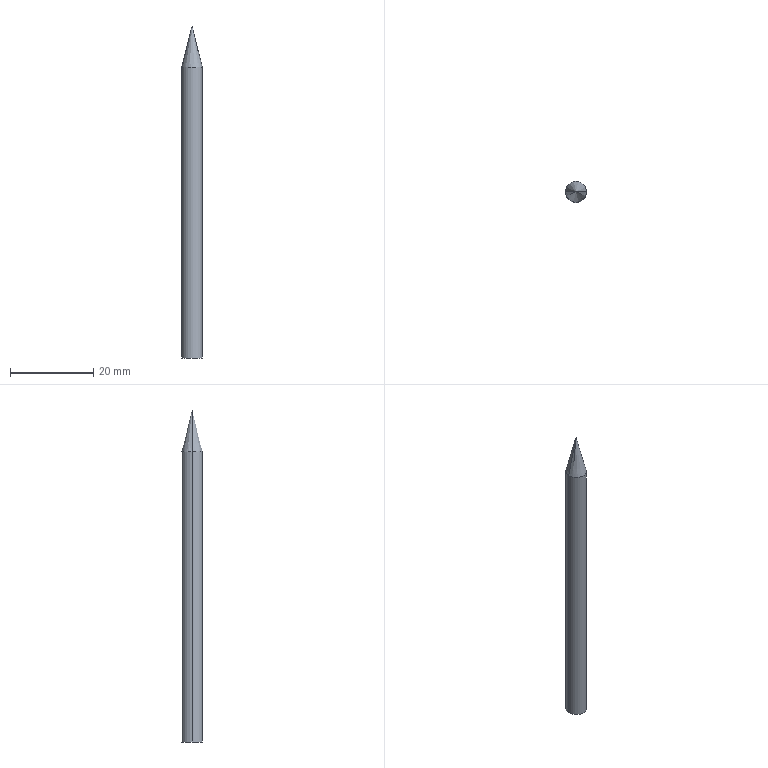Part | 1 solid | 5 faces | box 5 x 5 x 80 mm | volume 1440 mm3 | cone 2 | cylinder 2 | plane 1 | commonest cylinder face diameters 5 x2
STEP:
#1=CARTESIAN_POINT('',(0.,0.,80.));
#2=VERTEX_POINT('',#1);
#3=CARTESIAN_POINT('',(-2.5,0.,70.));
#4=VERTEX_POINT('',#3);
#5=CARTESIAN_POINT('',(0.,0.,80.));
#6=DIRECTION('',(-0.2425,0.,-0.9701));
#7=VECTOR('',#6,1000.);
#8=LINE('',#5,#7);
#9=EDGE_CURVE('',#2,#4,#8,.T.);
#10=ORIENTED_EDGE('',*,*,#9,.F.);
#11=CARTESIAN_POINT('',(2.5,0.,70.));
#12=VERTEX_POINT('',#11);
#13=CARTESIAN_POINT('',(0.,0.,80.));
#14=DIRECTION('',(0.2425,0.,-0.9701));
#15=VECTOR('',#14,1000.);
#16=LINE('',#13,#15);
#17=EDGE_CURVE('',#2,#12,#16,.T.);
#18=ORIENTED_EDGE('',*,*,#17,.T.);
#19=CARTESIAN_POINT('',(0.,0.,70.));
#20=DIRECTION('',(0.,0.,-1.));
#21=DIRECTION('',(-1.,0.,0.));
#22=AXIS2_PLACEMENT_3D('',#19,#20,#21);
#23=CIRCLE('',#22,2.5);
#24=EDGE_CURVE('',#4,#12,#23,.T.);
#25=ORIENTED_EDGE('',*,*,#24,.F.);
#26=EDGE_LOOP('',(#10,#18,#25));
#27=FACE_OUTER_BOUND('',#26,.T.);
#28=CARTESIAN_POINT('',(0.,0.,-920.));
#29=DIRECTION('',(0.,0.,-1.));
#30=DIRECTION('',(-1.,0.,0.));
#31=AXIS2_PLACEMENT_3D('',#28,#29,#30);
#32=CONICAL_SURFACE('',#31,250.,0.245);
#33=ADVANCED_FACE('',(#27),#32,.T.);
#34=ORIENTED_EDGE('',*,*,#24,.T.);
#35=CARTESIAN_POINT('',(2.5,0.,0.));
#36=VERTEX_POINT('',#35);
#37=CARTESIAN_POINT('',(2.5,0.,80.));
#38=DIRECTION('',(0.,0.,-1.));
#39=VECTOR('',#38,1000.);
#40=LINE('',#37,#39);
#41=EDGE_CURVE('',#12,#36,#40,.T.);
#42=ORIENTED_EDGE('',*,*,#41,.T.);
#43=CARTESIAN_POINT('',(-2.5,0.,0.));
#44=VERTEX_POINT('',#43);
#45=CARTESIAN_POINT('',(0.,0.,0.));
#46=DIRECTION('',(0.,0.,1.));
#47=DIRECTION('',(1.,0.,0.));
#48=AXIS2_PLACEMENT_3D('',#45,#46,#47);
#49=CIRCLE('',#48,2.5);
#50=EDGE_CURVE('',#36,#44,#49,.T.);
#51=ORIENTED_EDGE('',*,*,#50,.T.);
#52=CARTESIAN_POINT('',(-2.5,0.,80.));
#53=DIRECTION('',(0.,0.,-1.));
#54=VECTOR('',#53,1000.);
#55=LINE('',#52,#54);
#56=EDGE_CURVE('',#4,#44,#55,.T.);
#57=ORIENTED_EDGE('',*,*,#56,.F.);
#58=EDGE_LOOP('',(#34,#42,#51,#57));
#59=FACE_OUTER_BOUND('',#58,.T.);
#60=CARTESIAN_POINT('',(0.,0.,80.));
#61=DIRECTION('',(0.,0.,-1.));
#62=DIRECTION('',(-1.,0.,0.));
#63=AXIS2_PLACEMENT_3D('',#60,#61,#62);
#64=CYLINDRICAL_SURFACE('',#63,2.5);
#65=ADVANCED_FACE('',(#59),#64,.T.);
#66=ORIENTED_EDGE('',*,*,#41,.F.);
#67=CARTESIAN_POINT('',(0.,0.,70.));
#68=DIRECTION('',(0.,0.,-1.));
#69=DIRECTION('',(-1.,0.,0.));
#70=AXIS2_PLACEMENT_3D('',#67,#68,#69);
#71=CIRCLE('',#70,2.5);
#72=EDGE_CURVE('',#12,#4,#71,.T.);
#73=ORIENTED_EDGE('',*,*,#72,.T.);
#74=ORIENTED_EDGE('',*,*,#56,.T.);
#75=CARTESIAN_POINT('',(0.,0.,0.));
#76=DIRECTION('',(0.,0.,1.));
#77=DIRECTION('',(1.,0.,0.));
#78=AXIS2_PLACEMENT_3D('',#75,#76,#77);
#79=CIRCLE('',#78,2.5);
#80=EDGE_CURVE('',#44,#36,#79,.T.);
#81=ORIENTED_EDGE('',*,*,#80,.T.);
#82=EDGE_LOOP('',(#66,#73,#74,#81));
#83=FACE_OUTER_BOUND('',#82,.T.);
#84=CARTESIAN_POINT('',(0.,0.,80.));
#85=DIRECTION('',(0.,0.,-1.));
#86=DIRECTION('',(-1.,0.,0.));
#87=AXIS2_PLACEMENT_3D('',#84,#85,#86);
#88=CYLINDRICAL_SURFACE('',#87,2.5);
#89=ADVANCED_FACE('',(#83),#88,.T.);
#90=ORIENTED_EDGE('',*,*,#80,.F.);
#91=ORIENTED_EDGE('',*,*,#50,.F.);
#92=EDGE_LOOP('',(#90,#91));
#93=FACE_OUTER_BOUND('',#92,.T.);
#94=CARTESIAN_POINT('',(0.,0.,0.));
#95=DIRECTION('',(0.,0.,1.));
#96=DIRECTION('',(1.,0.,0.));
#97=AXIS2_PLACEMENT_3D('',#94,#95,#96);
#98=PLANE('',#97);
#99=ADVANCED_FACE('',(#93),#98,.F.);
#100=ORIENTED_EDGE('',*,*,#17,.F.);
#101=ORIENTED_EDGE('',*,*,#9,.T.);
#102=ORIENTED_EDGE('',*,*,#72,.F.);
#103=EDGE_LOOP('',(#100,#101,#102));
#104=FACE_OUTER_BOUND('',#103,.T.);
#105=CARTESIAN_POINT('',(0.,0.,-920.));
#106=DIRECTION('',(0.,0.,-1.));
#107=DIRECTION('',(-1.,0.,0.));
#108=AXIS2_PLACEMENT_3D('',#105,#106,#107);
#109=CONICAL_SURFACE('',#108,250.,0.245);
#110=ADVANCED_FACE('',(#104),#109,.T.);
#111=CLOSED_SHELL('',(#33,#65,#89,#99,#110));
#112=MANIFOLD_SOLID_BREP('',#111);
#113=CARTESIAN_POINT('',(0.,0.,0.));
#114=DIRECTION('',(0.,0.,1.));
#115=DIRECTION('',(1.,0.,0.));
#116=AXIS2_PLACEMENT_3D('',#113,#114,#115);
#117=(LENGTH_UNIT()NAMED_UNIT(*)SI_UNIT(.MILLI.,.METRE.));
#118=UNCERTAINTY_MEASURE_WITH_UNIT(LENGTH_MEASURE(0.00001),#117,'','');
#119=(NAMED_UNIT(*)PLANE_ANGLE_UNIT()SI_UNIT($,.RADIAN.));
#120=(NAMED_UNIT(*)SI_UNIT($,.STERADIAN.)SOLID_ANGLE_UNIT());
#121=(GEOMETRIC_REPRESENTATION_CONTEXT(3)GLOBAL_UNCERTAINTY_ASSIGNED_CONTEXT((#118))GLOBAL_UNIT_ASSIGNED_CONTEXT((#117,#119,#120))REPRESENTATION_CONTEXT('',''));
#122=ADVANCED_BREP_SHAPE_REPRESENTATION('',(#112,#116),#121);